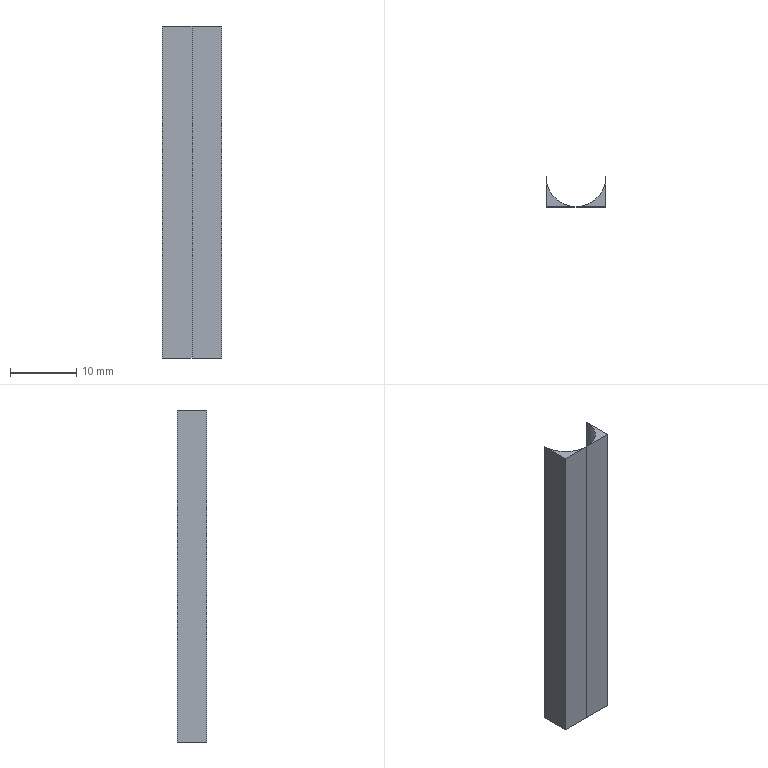Part | STEP file | DCV-000-W02_1 | 2 solids | 10 faces | box 9 x 4.5 x 50 mm | volume 434.569 mm3 | plane 8 | cylinder 2 | commonest cylinder face diameters 9 x2
STEP:
#1=CARTESIAN_POINT('',(0.,0.,0.));
#2=DIRECTION('',(0.,0.,1.));
#3=DIRECTION('',(1.,0.,0.));
#4=AXIS2_PLACEMENT_3D('',#1,#2,#3);
#5=CARTESIAN_POINT('',(0.,-4.5,220.));
#6=VERTEX_POINT('',#5);
#7=CARTESIAN_POINT('',(4.5,0.,220.));
#8=VERTEX_POINT('',#7);
#9=CARTESIAN_POINT('',(0.,0.,220.));
#10=DIRECTION('',(0.,0.,1.));
#11=DIRECTION('',(1.,0.,0.));
#12=AXIS2_PLACEMENT_3D('',#9,#10,#11);
#13=CIRCLE('',#12,4.5);
#14=CARTESIAN_POINT('',(10.5,-4.5,220.));
#15=DIRECTION('',(0.,0.,1.));
#16=DIRECTION('',(1.,0.,0.));
#17=AXIS2_PLACEMENT_3D('',#14,#15,#16);
#18=PLANE('',#17);
#19=CARTESIAN_POINT('',(-10.5,4.5));
#20=DIRECTION('',(1.,0.));
#21=AXIS2_PLACEMENT_2D('',#19,#20);
#22=CIRCLE('',#21,4.5);
#23=(GEOMETRIC_REPRESENTATION_CONTEXT(2)PARAMETRIC_REPRESENTATION_CONTEXT()REPRESENTATION_CONTEXT('',''));
#24=DEFINITIONAL_REPRESENTATION('',(#22),#23);
#25=PCURVE('',#18,#24);
#26=CARTESIAN_POINT('',(0.,0.,0.));
#27=DIRECTION('',(0.,0.,1.));
#28=DIRECTION('',(1.,0.,0.));
#29=AXIS2_PLACEMENT_3D('',#26,#27,#28);
#30=CYLINDRICAL_SURFACE('',#29,4.5);
#31=CARTESIAN_POINT('',(0.,220.));
#32=DIRECTION('',(1.,0.));
#33=VECTOR('',#32,1.);
#34=LINE('',#31,#33);
#35=(GEOMETRIC_REPRESENTATION_CONTEXT(2)PARAMETRIC_REPRESENTATION_CONTEXT()REPRESENTATION_CONTEXT('',''));
#36=DEFINITIONAL_REPRESENTATION('',(#34),#35);
#37=PCURVE('',#30,#36);
#38=SURFACE_CURVE('',#13,(#25,#37),.PCURVE_S1.);
#39=EDGE_CURVE('',#6,#8,#38,.T.);
#40=ORIENTED_EDGE('',*,*,#39,.F.);
#41=CARTESIAN_POINT('',(4.5,-4.5,220.));
#42=VERTEX_POINT('',#41);
#43=CARTESIAN_POINT('',(0.,-4.5,220.));
#44=DIRECTION('',(1.,0.,0.));
#45=VECTOR('',#44,1.);
#46=LINE('',#43,#45);
#47=CARTESIAN_POINT('',(-10.5,0.));
#48=DIRECTION('',(1.,0.));
#49=VECTOR('',#48,1.);
#50=LINE('',#47,#49);
#51=(GEOMETRIC_REPRESENTATION_CONTEXT(2)PARAMETRIC_REPRESENTATION_CONTEXT()REPRESENTATION_CONTEXT('',''));
#52=DEFINITIONAL_REPRESENTATION('',(#50),#51);
#53=PCURVE('',#18,#52);
#54=CARTESIAN_POINT('',(0.,-4.5,197.5));
#55=DIRECTION('',(0.,-1.,0.));
#56=DIRECTION('',(0.,0.,-1.));
#57=AXIS2_PLACEMENT_3D('',#54,#55,#56);
#58=PLANE('',#57);
#59=CARTESIAN_POINT('',(-22.5,0.));
#60=DIRECTION('',(0.,1.));
#61=VECTOR('',#60,1.);
#62=LINE('',#59,#61);
#63=(GEOMETRIC_REPRESENTATION_CONTEXT(2)PARAMETRIC_REPRESENTATION_CONTEXT()REPRESENTATION_CONTEXT('',''));
#64=DEFINITIONAL_REPRESENTATION('',(#62),#63);
#65=PCURVE('',#58,#64);
#66=SURFACE_CURVE('',#46,(#53,#65),.PCURVE_S1.);
#67=EDGE_CURVE('',#6,#42,#66,.T.);
#68=ORIENTED_EDGE('',*,*,#67,.T.);
#69=CARTESIAN_POINT('',(4.5,-2.25,220.));
#70=DIRECTION('',(0.,-1.,0.));
#71=VECTOR('',#70,1.);
#72=LINE('',#69,#71);
#73=CARTESIAN_POINT('',(-6.,2.25));
#74=DIRECTION('',(0.,-1.));
#75=VECTOR('',#74,1.);
#76=LINE('',#73,#75);
#77=(GEOMETRIC_REPRESENTATION_CONTEXT(2)PARAMETRIC_REPRESENTATION_CONTEXT()REPRESENTATION_CONTEXT('',''));
#78=DEFINITIONAL_REPRESENTATION('',(#76),#77);
#79=PCURVE('',#18,#78);
#80=CARTESIAN_POINT('',(4.5,0.,0.));
#81=DIRECTION('',(1.,0.,0.));
#82=DIRECTION('',(0.,1.,0.));
#83=AXIS2_PLACEMENT_3D('',#80,#81,#82);
#84=PLANE('',#83);
#85=CARTESIAN_POINT('',(-2.25,220.));
#86=DIRECTION('',(-1.,0.));
#87=VECTOR('',#86,1.);
#88=LINE('',#85,#87);
#89=(GEOMETRIC_REPRESENTATION_CONTEXT(2)PARAMETRIC_REPRESENTATION_CONTEXT()REPRESENTATION_CONTEXT('',''));
#90=DEFINITIONAL_REPRESENTATION('',(#88),#89);
#91=PCURVE('',#84,#90);
#92=SURFACE_CURVE('',#72,(#79,#91),.PCURVE_S1.);
#93=EDGE_CURVE('',#8,#42,#92,.T.);
#94=ORIENTED_EDGE('',*,*,#93,.F.);
#95=EDGE_LOOP('',(#40,#68,#94));
#96=FACE_BOUND('',#95,.T.);
#97=ADVANCED_FACE('',(#96),#18,.T.);
#98=CARTESIAN_POINT('',(4.5,-4.5,170.));
#99=VERTEX_POINT('',#98);
#100=CARTESIAN_POINT('',(4.5,-4.5,98.75));
#101=DIRECTION('',(0.,0.,-1.));
#102=VECTOR('',#101,1.);
#103=LINE('',#100,#102);
#104=CARTESIAN_POINT('',(98.75,4.5));
#105=DIRECTION('',(1.,0.));
#106=VECTOR('',#105,1.);
#107=LINE('',#104,#106);
#108=(GEOMETRIC_REPRESENTATION_CONTEXT(2)PARAMETRIC_REPRESENTATION_CONTEXT()REPRESENTATION_CONTEXT('',''));
#109=DEFINITIONAL_REPRESENTATION('',(#107),#108);
#110=PCURVE('',#58,#109);
#111=CARTESIAN_POINT('',(-4.5,98.75));
#112=DIRECTION('',(0.,-1.));
#113=VECTOR('',#112,1.);
#114=LINE('',#111,#113);
#115=(GEOMETRIC_REPRESENTATION_CONTEXT(2)PARAMETRIC_REPRESENTATION_CONTEXT()REPRESENTATION_CONTEXT('',''));
#116=DEFINITIONAL_REPRESENTATION('',(#114),#115);
#117=PCURVE('',#84,#116);
#118=SURFACE_CURVE('',#103,(#110,#117),.PCURVE_S1.);
#119=EDGE_CURVE('',#42,#99,#118,.T.);
#120=ORIENTED_EDGE('',*,*,#119,.F.);
#121=ORIENTED_EDGE('',*,*,#67,.F.);
#122=CARTESIAN_POINT('',(0.,-4.5,170.));
#123=VERTEX_POINT('',#122);
#124=CARTESIAN_POINT('',(0.,-4.5,0.));
#125=DIRECTION('',(0.,0.,1.));
#126=VECTOR('',#125,1.);
#127=LINE('',#124,#126);
#128=CARTESIAN_POINT('',(197.5,0.));
#129=DIRECTION('',(-1.,0.));
#130=VECTOR('',#129,1.);
#131=LINE('',#128,#130);
#132=(GEOMETRIC_REPRESENTATION_CONTEXT(2)PARAMETRIC_REPRESENTATION_CONTEXT()REPRESENTATION_CONTEXT('',''));
#133=DEFINITIONAL_REPRESENTATION('',(#131),#132);
#134=PCURVE('',#58,#133);
#135=CARTESIAN_POINT('',(4.712,0.));
#136=DIRECTION('',(0.,1.));
#137=VECTOR('',#136,1.);
#138=LINE('',#135,#137);
#139=(GEOMETRIC_REPRESENTATION_CONTEXT(2)PARAMETRIC_REPRESENTATION_CONTEXT()REPRESENTATION_CONTEXT('',''));
#140=DEFINITIONAL_REPRESENTATION('',(#138),#139);
#141=PCURVE('',#30,#140);
#142=SURFACE_CURVE('',#127,(#134,#141),.PCURVE_S1.);
#143=EDGE_CURVE('',#123,#6,#142,.T.);
#144=ORIENTED_EDGE('',*,*,#143,.F.);
#145=CARTESIAN_POINT('',(-17.5,-4.5,170.));
#146=DIRECTION('',(1.,0.,0.));
#147=VECTOR('',#146,1.);
#148=LINE('',#145,#147);
#149=CARTESIAN_POINT('',(27.5,-17.5));
#150=DIRECTION('',(0.,1.));
#151=VECTOR('',#150,1.);
#152=LINE('',#149,#151);
#153=(GEOMETRIC_REPRESENTATION_CONTEXT(2)PARAMETRIC_REPRESENTATION_CONTEXT()REPRESENTATION_CONTEXT('',''));
#154=DEFINITIONAL_REPRESENTATION('',(#152),#153);
#155=PCURVE('',#58,#154);
#156=CARTESIAN_POINT('',(0.,-4.5,170.));
#157=DIRECTION('',(0.,0.,-1.));
#158=DIRECTION('',(0.,-1.,0.));
#159=AXIS2_PLACEMENT_3D('',#156,#157,#158);
#160=PLANE('',#159);
#161=CARTESIAN_POINT('',(0.,17.5));
#162=DIRECTION('',(0.,-1.));
#163=VECTOR('',#162,1.);
#164=LINE('',#161,#163);
#165=(GEOMETRIC_REPRESENTATION_CONTEXT(2)PARAMETRIC_REPRESENTATION_CONTEXT()REPRESENTATION_CONTEXT('',''));
#166=DEFINITIONAL_REPRESENTATION('',(#164),#165);
#167=PCURVE('',#160,#166);
#168=SURFACE_CURVE('',#148,(#155,#167),.PCURVE_S1.);
#169=EDGE_CURVE('',#123,#99,#168,.T.);
#170=ORIENTED_EDGE('',*,*,#169,.T.);
#171=EDGE_LOOP('',(#120,#121,#144,#170));
#172=FACE_BOUND('',#171,.T.);
#173=ADVANCED_FACE('',(#172),#58,.T.);
#174=CARTESIAN_POINT('',(4.5,0.,170.));
#175=VERTEX_POINT('',#174);
#176=CARTESIAN_POINT('',(0.,0.,170.));
#177=DIRECTION('',(0.,0.,-1.));
#178=DIRECTION('',(1.,0.,0.));
#179=AXIS2_PLACEMENT_3D('',#176,#177,#178);
#180=CIRCLE('',#179,4.5);
#181=CARTESIAN_POINT('',(-4.5,0.));
#182=DIRECTION('',(0.,-1.));
#183=AXIS2_PLACEMENT_2D('',#181,#182);
#184=CIRCLE('',#183,4.5);
#185=(GEOMETRIC_REPRESENTATION_CONTEXT(2)PARAMETRIC_REPRESENTATION_CONTEXT()REPRESENTATION_CONTEXT('',''));
#186=DEFINITIONAL_REPRESENTATION('',(#184),#185);
#187=PCURVE('',#160,#186);
#188=CARTESIAN_POINT('',(6.283,170.));
#189=DIRECTION('',(-1.,0.));
#190=VECTOR('',#189,1.);
#191=LINE('',#188,#190);
#192=(GEOMETRIC_REPRESENTATION_CONTEXT(2)PARAMETRIC_REPRESENTATION_CONTEXT()REPRESENTATION_CONTEXT('',''));
#193=DEFINITIONAL_REPRESENTATION('',(#191),#192);
#194=PCURVE('',#30,#193);
#195=SURFACE_CURVE('',#180,(#187,#194),.PCURVE_S1.);
#196=EDGE_CURVE('',#175,#123,#195,.T.);
#197=ORIENTED_EDGE('',*,*,#196,.F.);
#198=CARTESIAN_POINT('',(4.5,-2.25,170.));
#199=DIRECTION('',(0.,1.,0.));
#200=VECTOR('',#199,1.);
#201=LINE('',#198,#200);
#202=CARTESIAN_POINT('',(-2.25,-4.5));
#203=DIRECTION('',(-1.,0.));
#204=VECTOR('',#203,1.);
#205=LINE('',#202,#204);
#206=(GEOMETRIC_REPRESENTATION_CONTEXT(2)PARAMETRIC_REPRESENTATION_CONTEXT()REPRESENTATION_CONTEXT('',''));
#207=DEFINITIONAL_REPRESENTATION('',(#205),#206);
#208=PCURVE('',#160,#207);
#209=CARTESIAN_POINT('',(-2.25,170.));
#210=DIRECTION('',(1.,0.));
#211=VECTOR('',#210,1.);
#212=LINE('',#209,#211);
#213=(GEOMETRIC_REPRESENTATION_CONTEXT(2)PARAMETRIC_REPRESENTATION_CONTEXT()REPRESENTATION_CONTEXT('',''));
#214=DEFINITIONAL_REPRESENTATION('',(#212),#213);
#215=PCURVE('',#84,#214);
#216=SURFACE_CURVE('',#201,(#208,#215),.PCURVE_S1.);
#217=EDGE_CURVE('',#99,#175,#216,.T.);
#218=ORIENTED_EDGE('',*,*,#217,.F.);
#219=ORIENTED_EDGE('',*,*,#169,.F.);
#220=EDGE_LOOP('',(#197,#218,#219));
#221=FACE_BOUND('',#220,.T.);
#222=ADVANCED_FACE('',(#221),#160,.T.);
#223=ORIENTED_EDGE('',*,*,#217,.T.);
#224=CARTESIAN_POINT('',(4.5,0.,0.));
#225=DIRECTION('',(0.,0.,1.));
#226=VECTOR('',#225,1.);
#227=LINE('',#224,#226);
#228=CARTESIAN_POINT('',(0.,0.));
#229=DIRECTION('',(0.,1.));
#230=VECTOR('',#229,1.);
#231=LINE('',#228,#230);
#232=(GEOMETRIC_REPRESENTATION_CONTEXT(2)PARAMETRIC_REPRESENTATION_CONTEXT()REPRESENTATION_CONTEXT('',''));
#233=DEFINITIONAL_REPRESENTATION('',(#231),#232);
#234=PCURVE('',#84,#233);
#235=CARTESIAN_POINT('',(6.283,0.));
#236=DIRECTION('',(0.,1.));
#237=VECTOR('',#236,1.);
#238=LINE('',#235,#237);
#239=(GEOMETRIC_REPRESENTATION_CONTEXT(2)PARAMETRIC_REPRESENTATION_CONTEXT()REPRESENTATION_CONTEXT('',''));
#240=DEFINITIONAL_REPRESENTATION('',(#238),#239);
#241=PCURVE('',#30,#240);
#242=SURFACE_CURVE('',#227,(#234,#241),.PCURVE_S1.);
#243=EDGE_CURVE('',#175,#8,#242,.T.);
#244=ORIENTED_EDGE('',*,*,#243,.T.);
#245=ORIENTED_EDGE('',*,*,#93,.T.);
#246=ORIENTED_EDGE('',*,*,#119,.T.);
#247=EDGE_LOOP('',(#223,#244,#245,#246));
#248=FACE_BOUND('',#247,.T.);
#249=ADVANCED_FACE('',(#248),#84,.T.);
#250=ORIENTED_EDGE('',*,*,#243,.T.);
#251=ORIENTED_EDGE('',*,*,#39,.F.);
#252=ORIENTED_EDGE('',*,*,#143,.F.);
#253=ORIENTED_EDGE('',*,*,#196,.F.);
#254=EDGE_LOOP('',(#250,#251,#252,#253));
#255=FACE_BOUND('',#254,.F.);
#256=ADVANCED_FACE('',(#255),#30,.F.);
#257=CLOSED_SHELL('',(#97,#173,#222,#249,#256));
#258=MANIFOLD_SOLID_BREP('',#257);
#259=CARTESIAN_POINT('',(-4.5,0.,220.));
#260=VERTEX_POINT('',#259);
#261=CARTESIAN_POINT('',(0.,-4.5,220.));
#262=VERTEX_POINT('',#261);
#263=CARTESIAN_POINT('',(0.,0.,220.));
#264=DIRECTION('',(0.,0.,1.));
#265=DIRECTION('',(1.,0.,0.));
#266=AXIS2_PLACEMENT_3D('',#263,#264,#265);
#267=CIRCLE('',#266,4.5);
#268=CARTESIAN_POINT('',(0.,0.,0.));
#269=DIRECTION('',(0.,0.,1.));
#270=DIRECTION('',(1.,0.,0.));
#271=AXIS2_PLACEMENT_3D('',#268,#269,#270);
#272=CYLINDRICAL_SURFACE('',#271,4.5);
#273=CARTESIAN_POINT('',(0.,220.));
#274=DIRECTION('',(1.,0.));
#275=VECTOR('',#274,1.);
#276=LINE('',#273,#275);
#277=(GEOMETRIC_REPRESENTATION_CONTEXT(2)PARAMETRIC_REPRESENTATION_CONTEXT()REPRESENTATION_CONTEXT('',''));
#278=DEFINITIONAL_REPRESENTATION('',(#276),#277);
#279=PCURVE('',#272,#278);
#280=CARTESIAN_POINT('',(0.,-4.5,220.));
#281=DIRECTION('',(0.,0.,1.));
#282=DIRECTION('',(1.,0.,0.));
#283=AXIS2_PLACEMENT_3D('',#280,#281,#282);
#284=PLANE('',#283);
#285=CARTESIAN_POINT('',(0.,4.5));
#286=DIRECTION('',(1.,0.));
#287=AXIS2_PLACEMENT_2D('',#285,#286);
#288=CIRCLE('',#287,4.5);
#289=(GEOMETRIC_REPRESENTATION_CONTEXT(2)PARAMETRIC_REPRESENTATION_CONTEXT()REPRESENTATION_CONTEXT('',''));
#290=DEFINITIONAL_REPRESENTATION('',(#288),#289);
#291=PCURVE('',#284,#290);
#292=SURFACE_CURVE('',#267,(#279,#291),.PCURVE_S1.);
#293=EDGE_CURVE('',#260,#262,#292,.T.);
#294=ORIENTED_EDGE('',*,*,#293,.F.);
#295=CARTESIAN_POINT('',(-4.5,0.,170.));
#296=VERTEX_POINT('',#295);
#297=CARTESIAN_POINT('',(-4.5,0.,0.));
#298=DIRECTION('',(0.,0.,-1.));
#299=VECTOR('',#298,1.);
#300=LINE('',#297,#299);
#301=CARTESIAN_POINT('',(3.142,0.));
#302=DIRECTION('',(0.,-1.));
#303=VECTOR('',#302,1.);
#304=LINE('',#301,#303);
#305=(GEOMETRIC_REPRESENTATION_CONTEXT(2)PARAMETRIC_REPRESENTATION_CONTEXT()REPRESENTATION_CONTEXT('',''));
#306=DEFINITIONAL_REPRESENTATION('',(#304),#305);
#307=PCURVE('',#272,#306);
#308=CARTESIAN_POINT('',(-4.5,0.,220.));
#309=DIRECTION('',(-1.,0.,0.));
#310=DIRECTION('',(0.,0.,1.));
#311=AXIS2_PLACEMENT_3D('',#308,#309,#310);
#312=PLANE('',#311);
#313=CARTESIAN_POINT('',(-220.,0.));
#314=DIRECTION('',(-1.,0.));
#315=VECTOR('',#314,1.);
#316=LINE('',#313,#315);
#317=(GEOMETRIC_REPRESENTATION_CONTEXT(2)PARAMETRIC_REPRESENTATION_CONTEXT()REPRESENTATION_CONTEXT('',''));
#318=DEFINITIONAL_REPRESENTATION('',(#316),#317);
#319=PCURVE('',#312,#318);
#320=SURFACE_CURVE('',#300,(#307,#319),.PCURVE_S1.);
#321=EDGE_CURVE('',#260,#296,#320,.T.);
#322=ORIENTED_EDGE('',*,*,#321,.T.);
#323=CARTESIAN_POINT('',(0.,-4.5,170.));
#324=VERTEX_POINT('',#323);
#325=CARTESIAN_POINT('',(0.,0.,170.));
#326=DIRECTION('',(0.,0.,-1.));
#327=DIRECTION('',(1.,0.,0.));
#328=AXIS2_PLACEMENT_3D('',#325,#326,#327);
#329=CIRCLE('',#328,4.5);
#330=CARTESIAN_POINT('',(6.283,170.));
#331=DIRECTION('',(-1.,0.));
#332=VECTOR('',#331,1.);
#333=LINE('',#330,#332);
#334=(GEOMETRIC_REPRESENTATION_CONTEXT(2)PARAMETRIC_REPRESENTATION_CONTEXT()REPRESENTATION_CONTEXT('',''));
#335=DEFINITIONAL_REPRESENTATION('',(#333),#334);
#336=PCURVE('',#272,#335);
#337=CARTESIAN_POINT('',(-12.5,-4.5,170.));
#338=DIRECTION('',(0.,0.,-1.));
#339=DIRECTION('',(0.,-1.,0.));
#340=AXIS2_PLACEMENT_3D('',#337,#338,#339);
#341=PLANE('',#340);
#342=CARTESIAN_POINT('',(-4.5,-12.5));
#343=DIRECTION('',(0.,-1.));
#344=AXIS2_PLACEMENT_2D('',#342,#343);
#345=CIRCLE('',#344,4.5);
#346=(GEOMETRIC_REPRESENTATION_CONTEXT(2)PARAMETRIC_REPRESENTATION_CONTEXT()REPRESENTATION_CONTEXT('',''));
#347=DEFINITIONAL_REPRESENTATION('',(#345),#346);
#348=PCURVE('',#341,#347);
#349=SURFACE_CURVE('',#329,(#336,#348),.PCURVE_S1.);
#350=EDGE_CURVE('',#324,#296,#349,.T.);
#351=ORIENTED_EDGE('',*,*,#350,.F.);
#352=CARTESIAN_POINT('',(0.,-4.5,0.));
#353=DIRECTION('',(0.,0.,1.));
#354=VECTOR('',#353,1.);
#355=LINE('',#352,#354);
#356=CARTESIAN_POINT('',(4.712,0.));
#357=DIRECTION('',(0.,1.));
#358=VECTOR('',#357,1.);
#359=LINE('',#356,#358);
#360=(GEOMETRIC_REPRESENTATION_CONTEXT(2)PARAMETRIC_REPRESENTATION_CONTEXT()REPRESENTATION_CONTEXT('',''));
#361=DEFINITIONAL_REPRESENTATION('',(#359),#360);
#362=PCURVE('',#272,#361);
#363=CARTESIAN_POINT('',(0.,-4.5,197.5));
#364=DIRECTION('',(0.,-1.,0.));
#365=DIRECTION('',(0.,0.,-1.));
#366=AXIS2_PLACEMENT_3D('',#363,#364,#365);
#367=PLANE('',#366);
#368=CARTESIAN_POINT('',(197.5,0.));
#369=DIRECTION('',(-1.,0.));
#370=VECTOR('',#369,1.);
#371=LINE('',#368,#370);
#372=(GEOMETRIC_REPRESENTATION_CONTEXT(2)PARAMETRIC_REPRESENTATION_CONTEXT()REPRESENTATION_CONTEXT('',''));
#373=DEFINITIONAL_REPRESENTATION('',(#371),#372);
#374=PCURVE('',#367,#373);
#375=SURFACE_CURVE('',#355,(#362,#374),.PCURVE_S1.);
#376=EDGE_CURVE('',#324,#262,#375,.T.);
#377=ORIENTED_EDGE('',*,*,#376,.T.);
#378=EDGE_LOOP('',(#294,#322,#351,#377));
#379=FACE_BOUND('',#378,.F.);
#380=ADVANCED_FACE('',(#379),#272,.F.);
#381=CARTESIAN_POINT('',(-4.5,-4.5,170.));
#382=VERTEX_POINT('',#381);
#383=CARTESIAN_POINT('',(-4.5,-4.5,220.));
#384=VERTEX_POINT('',#383);
#385=CARTESIAN_POINT('',(-4.5,-4.5,208.75));
#386=DIRECTION('',(0.,0.,1.));
#387=VECTOR('',#386,1.);
#388=LINE('',#385,#387);
#389=CARTESIAN_POINT('',(-11.25,-4.5));
#390=DIRECTION('',(1.,0.));
#391=VECTOR('',#390,1.);
#392=LINE('',#389,#391);
#393=(GEOMETRIC_REPRESENTATION_CONTEXT(2)PARAMETRIC_REPRESENTATION_CONTEXT()REPRESENTATION_CONTEXT('',''));
#394=DEFINITIONAL_REPRESENTATION('',(#392),#393);
#395=PCURVE('',#312,#394);
#396=CARTESIAN_POINT('',(-11.25,-4.5));
#397=DIRECTION('',(-1.,0.));
#398=VECTOR('',#397,1.);
#399=LINE('',#396,#398);
#400=(GEOMETRIC_REPRESENTATION_CONTEXT(2)PARAMETRIC_REPRESENTATION_CONTEXT()REPRESENTATION_CONTEXT('',''));
#401=DEFINITIONAL_REPRESENTATION('',(#399),#400);
#402=PCURVE('',#367,#401);
#403=SURFACE_CURVE('',#388,(#395,#402),.PCURVE_S1.);
#404=EDGE_CURVE('',#382,#384,#403,.T.);
#405=ORIENTED_EDGE('',*,*,#404,.T.);
#406=CARTESIAN_POINT('',(-4.5,-2.25,220.));
#407=DIRECTION('',(0.,1.,0.));
#408=VECTOR('',#407,1.);
#409=LINE('',#406,#408);
#410=CARTESIAN_POINT('',(0.,-2.25));
#411=DIRECTION('',(0.,1.));
#412=VECTOR('',#411,1.);
#413=LINE('',#410,#412);
#414=(GEOMETRIC_REPRESENTATION_CONTEXT(2)PARAMETRIC_REPRESENTATION_CONTEXT()REPRESENTATION_CONTEXT('',''));
#415=DEFINITIONAL_REPRESENTATION('',(#413),#414);
#416=PCURVE('',#312,#415);
#417=CARTESIAN_POINT('',(-4.5,2.25));
#418=DIRECTION('',(0.,1.));
#419=VECTOR('',#418,1.);
#420=LINE('',#417,#419);
#421=(GEOMETRIC_REPRESENTATION_CONTEXT(2)PARAMETRIC_REPRESENTATION_CONTEXT()REPRESENTATION_CONTEXT('',''));
#422=DEFINITIONAL_REPRESENTATION('',(#420),#421);
#423=PCURVE('',#284,#422);
#424=SURFACE_CURVE('',#409,(#416,#423),.PCURVE_S1.);
#425=EDGE_CURVE('',#384,#260,#424,.T.);
#426=ORIENTED_EDGE('',*,*,#425,.T.);
#427=ORIENTED_EDGE('',*,*,#321,.T.);
#428=CARTESIAN_POINT('',(-4.5,-2.25,170.));
#429=DIRECTION('',(0.,-1.,0.));
#430=VECTOR('',#429,1.);
#431=LINE('',#428,#430);
#432=CARTESIAN_POINT('',(-50.,-2.25));
#433=DIRECTION('',(0.,-1.));
#434=VECTOR('',#433,1.);
#435=LINE('',#432,#434);
#436=(GEOMETRIC_REPRESENTATION_CONTEXT(2)PARAMETRIC_REPRESENTATION_CONTEXT()REPRESENTATION_CONTEXT('',''));
#437=DEFINITIONAL_REPRESENTATION('',(#435),#436);
#438=PCURVE('',#312,#437);
#439=CARTESIAN_POINT('',(-2.25,-8.));
#440=DIRECTION('',(1.,0.));
#441=VECTOR('',#440,1.);
#442=LINE('',#439,#441);
#443=(GEOMETRIC_REPRESENTATION_CONTEXT(2)PARAMETRIC_REPRESENTATION_CONTEXT()REPRESENTATION_CONTEXT('',''));
#444=DEFINITIONAL_REPRESENTATION('',(#442),#443);
#445=PCURVE('',#341,#444);
#446=SURFACE_CURVE('',#431,(#438,#445),.PCURVE_S1.);
#447=EDGE_CURVE('',#296,#382,#446,.T.);
#448=ORIENTED_EDGE('',*,*,#447,.T.);
#449=EDGE_LOOP('',(#405,#426,#427,#448));
#450=FACE_BOUND('',#449,.T.);
#451=ADVANCED_FACE('',(#450),#312,.T.);
#452=ORIENTED_EDGE('',*,*,#293,.F.);
#453=ORIENTED_EDGE('',*,*,#425,.F.);
#454=CARTESIAN_POINT('',(0.,-4.5,220.));
#455=DIRECTION('',(1.,0.,0.));
#456=VECTOR('',#455,1.);
#457=LINE('',#454,#456);
#458=CARTESIAN_POINT('',(0.,0.));
#459=DIRECTION('',(1.,0.));
#460=VECTOR('',#459,1.);
#461=LINE('',#458,#460);
#462=(GEOMETRIC_REPRESENTATION_CONTEXT(2)PARAMETRIC_REPRESENTATION_CONTEXT()REPRESENTATION_CONTEXT('',''));
#463=DEFINITIONAL_REPRESENTATION('',(#461),#462);
#464=PCURVE('',#284,#463);
#465=CARTESIAN_POINT('',(-22.5,0.));
#466=DIRECTION('',(0.,1.));
#467=VECTOR('',#466,1.);
#468=LINE('',#465,#467);
#469=(GEOMETRIC_REPRESENTATION_CONTEXT(2)PARAMETRIC_REPRESENTATION_CONTEXT()REPRESENTATION_CONTEXT('',''));
#470=DEFINITIONAL_REPRESENTATION('',(#468),#469);
#471=PCURVE('',#367,#470);
#472=SURFACE_CURVE('',#457,(#464,#471),.PCURVE_S1.);
#473=EDGE_CURVE('',#384,#262,#472,.T.);
#474=ORIENTED_EDGE('',*,*,#473,.T.);
#475=EDGE_LOOP('',(#452,#453,#474));
#476=FACE_BOUND('',#475,.T.);
#477=ADVANCED_FACE('',(#476),#284,.T.);
#478=ORIENTED_EDGE('',*,*,#404,.F.);
#479=CARTESIAN_POINT('',(-17.5,-4.5,170.));
#480=DIRECTION('',(1.,0.,0.));
#481=VECTOR('',#480,1.);
#482=LINE('',#479,#481);
#483=CARTESIAN_POINT('',(27.5,-17.5));
#484=DIRECTION('',(0.,1.));
#485=VECTOR('',#484,1.);
#486=LINE('',#483,#485);
#487=(GEOMETRIC_REPRESENTATION_CONTEXT(2)PARAMETRIC_REPRESENTATION_CONTEXT()REPRESENTATION_CONTEXT('',''));
#488=DEFINITIONAL_REPRESENTATION('',(#486),#487);
#489=PCURVE('',#367,#488);
#490=CARTESIAN_POINT('',(0.,5.));
#491=DIRECTION('',(0.,-1.));
#492=VECTOR('',#491,1.);
#493=LINE('',#490,#492);
#494=(GEOMETRIC_REPRESENTATION_CONTEXT(2)PARAMETRIC_REPRESENTATION_CONTEXT()REPRESENTATION_CONTEXT('',''));
#495=DEFINITIONAL_REPRESENTATION('',(#493),#494);
#496=PCURVE('',#341,#495);
#497=SURFACE_CURVE('',#482,(#489,#496),.PCURVE_S1.);
#498=EDGE_CURVE('',#382,#324,#497,.T.);
#499=ORIENTED_EDGE('',*,*,#498,.T.);
#500=ORIENTED_EDGE('',*,*,#376,.T.);
#501=ORIENTED_EDGE('',*,*,#473,.F.);
#502=EDGE_LOOP('',(#478,#499,#500,#501));
#503=FACE_BOUND('',#502,.T.);
#504=ADVANCED_FACE('',(#503),#367,.T.);
#505=ORIENTED_EDGE('',*,*,#350,.F.);
#506=ORIENTED_EDGE('',*,*,#498,.F.);
#507=ORIENTED_EDGE('',*,*,#447,.F.);
#508=EDGE_LOOP('',(#505,#506,#507));
#509=FACE_BOUND('',#508,.T.);
#510=ADVANCED_FACE('',(#509),#341,.T.);
#511=CLOSED_SHELL('',(#380,#451,#477,#504,#510));
#512=MANIFOLD_SOLID_BREP('',#511);
#513=(LENGTH_UNIT()NAMED_UNIT(*)SI_UNIT(.MILLI.,.METRE.));
#514=UNCERTAINTY_MEASURE_WITH_UNIT(LENGTH_MEASURE(0.0000001),#513,'','');
#515=(NAMED_UNIT(*)PLANE_ANGLE_UNIT()SI_UNIT($,.RADIAN.));
#516=(NAMED_UNIT(*)SI_UNIT($,.STERADIAN.)SOLID_ANGLE_UNIT());
#517=(GEOMETRIC_REPRESENTATION_CONTEXT(3)GLOBAL_UNCERTAINTY_ASSIGNED_CONTEXT((#514))GLOBAL_UNIT_ASSIGNED_CONTEXT((#513,#515,#516))REPRESENTATION_CONTEXT('',''));
#518=SHAPE_REPRESENTATION('',(#4,#258,#512),#517);